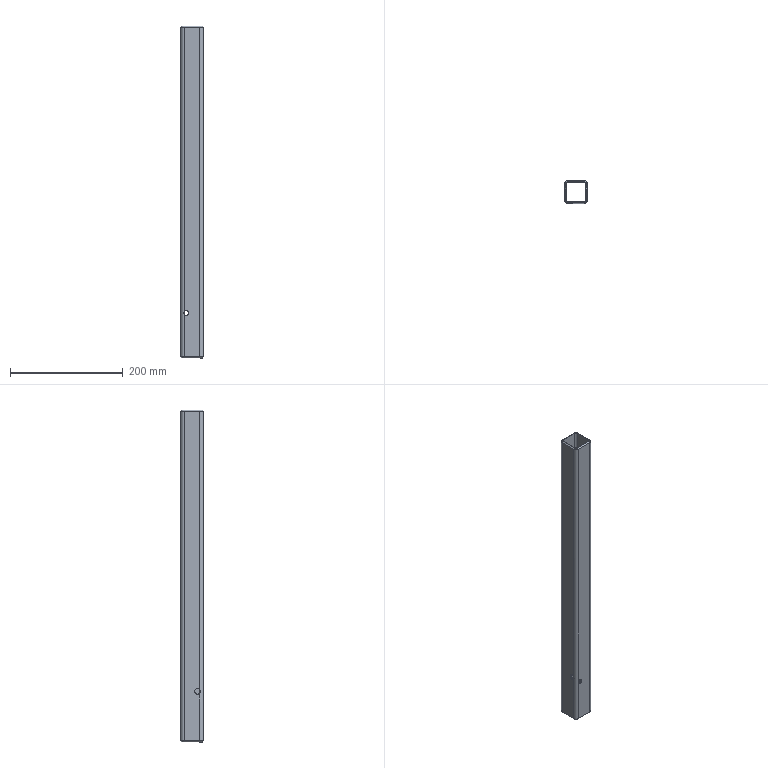Part | STEP file | IN-01-01-01-05 | 1 solid | 40 faces | box 40 x 40 x 590 mm | volume 239994 mm3 | plane 18 | cylinder 14 | cone 8 | commonest cylinder face diameters 5.8 x4 8.501 x4 11.6 x4 10 x2